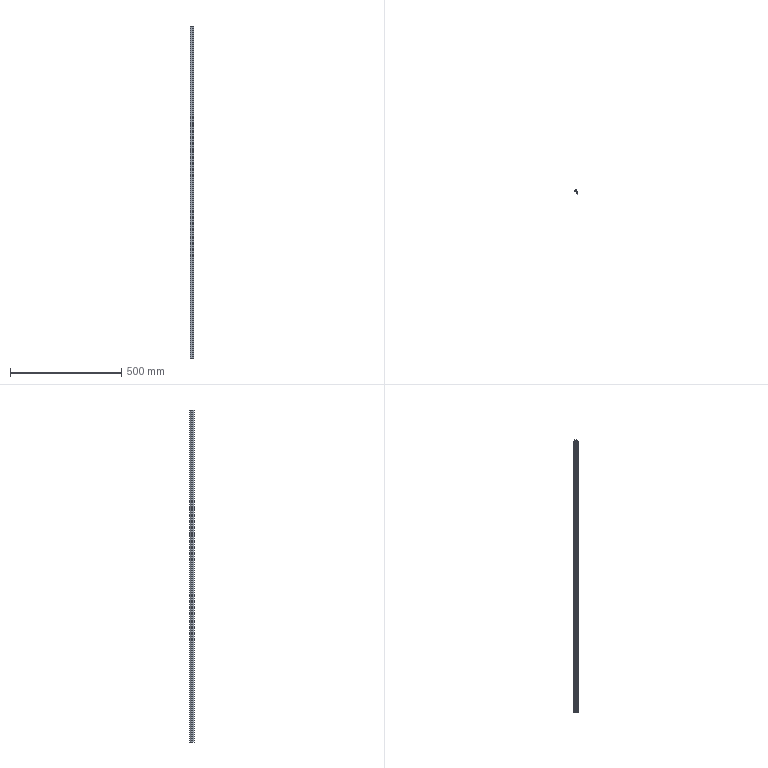Part | SolidWorks | features BaseBody 1, ICE 1, MoveFace 1 | 1 solid | 27 faces | box 14 x 20.3 x 1495 mm | volume 76119 mm3 | plane 20 | cylinder 7 | commonest cylinder face diameters 0.387 x2 0.8 x2 0.4 x1 20 x1 22 x1
STEP:
#1=CARTESIAN_POINT('',(-5.304,-0.625,200.));
#2=VERTEX_POINT('',#1);
#3=CARTESIAN_POINT('',(-5.449,-0.8125,200.));
#4=VERTEX_POINT('',#3);
#5=CARTESIAN_POINT('',(-5.255,-0.8125,200.));
#6=DIRECTION('',(0.,0.,1.));
#7=DIRECTION('',(-1.,0.,0.));
#8=AXIS2_PLACEMENT_3D('',#5,#6,#7);
#9=CIRCLE('',#8,0.1937);
#10=EDGE_CURVE('',#2,#4,#9,.T.);
#11=ORIENTED_EDGE('',*,*,#10,.T.);
#12=CARTESIAN_POINT('',(-5.449,-0.8125,-1295.));
#13=VERTEX_POINT('',#12);
#14=CARTESIAN_POINT('',(-5.449,-0.8125,230.));
#15=DIRECTION('',(0.,0.,-1.));
#16=VECTOR('',#15,1000.);
#17=LINE('',#14,#16);
#18=EDGE_CURVE('',#4,#13,#17,.T.);
#19=ORIENTED_EDGE('',*,*,#18,.T.);
#20=CARTESIAN_POINT('',(-5.304,-0.625,-1295.));
#21=VERTEX_POINT('',#20);
#22=CARTESIAN_POINT('',(-5.255,-0.8125,-1295.));
#23=DIRECTION('',(0.,0.,-1.));
#24=DIRECTION('',(1.,0.,0.));
#25=AXIS2_PLACEMENT_3D('',#22,#23,#24);
#26=CIRCLE('',#25,0.1937);
#27=EDGE_CURVE('',#13,#21,#26,.T.);
#28=ORIENTED_EDGE('',*,*,#27,.T.);
#29=CARTESIAN_POINT('',(-5.304,-0.625,230.));
#30=DIRECTION('',(0.,0.,-1.));
#31=VECTOR('',#30,1000.);
#32=LINE('',#29,#31);
#33=EDGE_CURVE('',#2,#21,#32,.T.);
#34=ORIENTED_EDGE('',*,*,#33,.F.);
#35=EDGE_LOOP('',(#11,#19,#28,#34));
#36=FACE_OUTER_BOUND('',#35,.T.);
#37=CARTESIAN_POINT('',(-5.255,-0.8125,230.));
#38=DIRECTION('',(0.,0.,-1.));
#39=DIRECTION('',(-1.,0.,0.));
#40=AXIS2_PLACEMENT_3D('',#37,#38,#39);
#41=CYLINDRICAL_SURFACE('',#40,0.1937);
#42=ADVANCED_FACE('',(#36),#41,.F.);
#43=CARTESIAN_POINT('',(5.,-1.,-1295.));
#44=VERTEX_POINT('',#43);
#45=CARTESIAN_POINT('',(5.,-14.3,-1295.));
#46=VERTEX_POINT('',#45);
#47=CARTESIAN_POINT('',(5.,29.623,-1295.));
#48=DIRECTION('',(0.,-1.,0.));
#49=VECTOR('',#48,1000.);
#50=LINE('',#47,#49);
#51=EDGE_CURVE('',#44,#46,#50,.T.);
#52=ORIENTED_EDGE('',*,*,#51,.F.);
#53=CARTESIAN_POINT('',(5.,-1.,200.));
#54=VERTEX_POINT('',#53);
#55=CARTESIAN_POINT('',(5.,-1.,230.));
#56=DIRECTION('',(0.,0.,-1.));
#57=VECTOR('',#56,1000.);
#58=LINE('',#55,#57);
#59=EDGE_CURVE('',#54,#44,#58,.T.);
#60=ORIENTED_EDGE('',*,*,#59,.F.);
#61=CARTESIAN_POINT('',(5.,-14.3,200.));
#62=VERTEX_POINT('',#61);
#63=CARTESIAN_POINT('',(5.,-14.3,200.));
#64=DIRECTION('',(0.,1.,0.));
#65=VECTOR('',#64,1000.);
#66=LINE('',#63,#65);
#67=EDGE_CURVE('',#62,#54,#66,.T.);
#68=ORIENTED_EDGE('',*,*,#67,.F.);
#69=CARTESIAN_POINT('',(5.,-14.3,230.));
#70=DIRECTION('',(0.,0.,1.));
#71=VECTOR('',#70,1000.);
#72=LINE('',#69,#71);
#73=EDGE_CURVE('',#46,#62,#72,.T.);
#74=ORIENTED_EDGE('',*,*,#73,.F.);
#75=EDGE_LOOP('',(#52,#60,#68,#74));
#76=FACE_OUTER_BOUND('',#75,.T.);
#77=CARTESIAN_POINT('',(5.,-14.3,230.));
#78=DIRECTION('',(-1.,0.,0.));
#79=DIRECTION('',(0.,0.,1.));
#80=AXIS2_PLACEMENT_3D('',#77,#78,#79);
#81=PLANE('',#80);
#82=ADVANCED_FACE('',(#76),#81,.F.);
#83=CARTESIAN_POINT('',(-9.,-2.,-1295.));
#84=VERTEX_POINT('',#83);
#85=CARTESIAN_POINT('',(-9.,-2.,200.));
#86=VERTEX_POINT('',#85);
#87=CARTESIAN_POINT('',(-9.,-2.,230.));
#88=DIRECTION('',(0.,0.,1.));
#89=VECTOR('',#88,1000.);
#90=LINE('',#87,#89);
#91=EDGE_CURVE('',#84,#86,#90,.T.);
#92=ORIENTED_EDGE('',*,*,#91,.F.);
#93=CARTESIAN_POINT('',(0.9,-2.,-1295.));
#94=VERTEX_POINT('',#93);
#95=CARTESIAN_POINT('',(5.,-2.,-1295.));
#96=DIRECTION('',(-1.,0.,0.));
#97=VECTOR('',#96,1000.);
#98=LINE('',#95,#97);
#99=EDGE_CURVE('',#94,#84,#98,.T.);
#100=ORIENTED_EDGE('',*,*,#99,.F.);
#101=CARTESIAN_POINT('',(0.9,-2.,200.));
#102=VERTEX_POINT('',#101);
#103=CARTESIAN_POINT('',(0.9,-2.,230.));
#104=DIRECTION('',(0.,0.,-1.));
#105=VECTOR('',#104,1000.);
#106=LINE('',#103,#105);
#107=EDGE_CURVE('',#102,#94,#106,.T.);
#108=ORIENTED_EDGE('',*,*,#107,.F.);
#109=CARTESIAN_POINT('',(5.,-2.,200.));
#110=DIRECTION('',(1.,0.,0.));
#111=VECTOR('',#110,1000.);
#112=LINE('',#109,#111);
#113=EDGE_CURVE('',#86,#102,#112,.T.);
#114=ORIENTED_EDGE('',*,*,#113,.F.);
#115=EDGE_LOOP('',(#92,#100,#108,#114));
#116=FACE_OUTER_BOUND('',#115,.T.);
#117=CARTESIAN_POINT('',(-9.,-2.,230.));
#118=DIRECTION('',(0.,1.,0.));
#119=DIRECTION('',(0.,0.,1.));
#120=AXIS2_PLACEMENT_3D('',#117,#118,#119);
#121=PLANE('',#120);
#122=ADVANCED_FACE('',(#116),#121,.F.);
#123=CARTESIAN_POINT('',(4.,-6.,200.));
#124=VERTEX_POINT('',#123);
#125=CARTESIAN_POINT('',(4.,-3.,200.));
#126=VERTEX_POINT('',#125);
#127=CARTESIAN_POINT('',(4.,29.623,200.));
#128=DIRECTION('',(0.,1.,0.));
#129=VECTOR('',#128,1000.);
#130=LINE('',#127,#129);
#131=EDGE_CURVE('',#124,#126,#130,.T.);
#132=ORIENTED_EDGE('',*,*,#131,.F.);
#133=CARTESIAN_POINT('',(1.,-6.,200.));
#134=VERTEX_POINT('',#133);
#135=CARTESIAN_POINT('',(5.,-6.,200.));
#136=DIRECTION('',(1.,0.,0.));
#137=VECTOR('',#136,1000.);
#138=LINE('',#135,#137);
#139=EDGE_CURVE('',#134,#124,#138,.T.);
#140=ORIENTED_EDGE('',*,*,#139,.F.);
#141=CARTESIAN_POINT('',(1.,-6.7,200.));
#142=VERTEX_POINT('',#141);
#143=CARTESIAN_POINT('',(1.,-6.,200.));
#144=DIRECTION('',(0.,-1.,0.));
#145=VECTOR('',#144,1000.);
#146=LINE('',#143,#145);
#147=EDGE_CURVE('',#134,#142,#146,.T.);
#148=ORIENTED_EDGE('',*,*,#147,.T.);
#149=CARTESIAN_POINT('',(-1.7,-6.7,200.));
#150=VERTEX_POINT('',#149);
#151=CARTESIAN_POINT('',(5.,-6.7,200.));
#152=DIRECTION('',(1.,0.,0.));
#153=VECTOR('',#152,1000.);
#154=LINE('',#151,#153);
#155=EDGE_CURVE('',#150,#142,#154,.T.);
#156=ORIENTED_EDGE('',*,*,#155,.F.);
#157=CARTESIAN_POINT('',(-1.7,-7.7,200.));
#158=VERTEX_POINT('',#157);
#159=CARTESIAN_POINT('',(-1.7,-6.7,200.));
#160=DIRECTION('',(0.,-1.,0.));
#161=VECTOR('',#160,1000.);
#162=LINE('',#159,#161);
#163=EDGE_CURVE('',#150,#158,#162,.T.);
#164=ORIENTED_EDGE('',*,*,#163,.T.);
#165=CARTESIAN_POINT('',(4.,-7.7,200.));
#166=VERTEX_POINT('',#165);
#167=CARTESIAN_POINT('',(5.,-7.7,200.));
#168=DIRECTION('',(-1.,0.,0.));
#169=VECTOR('',#168,1000.);
#170=LINE('',#167,#169);
#171=EDGE_CURVE('',#166,#158,#170,.T.);
#172=ORIENTED_EDGE('',*,*,#171,.F.);
#173=CARTESIAN_POINT('',(4.,-14.3,200.));
#174=VERTEX_POINT('',#173);
#175=CARTESIAN_POINT('',(4.,29.623,200.));
#176=DIRECTION('',(0.,1.,0.));
#177=VECTOR('',#176,1000.);
#178=LINE('',#175,#177);
#179=EDGE_CURVE('',#174,#166,#178,.T.);
#180=ORIENTED_EDGE('',*,*,#179,.F.);
#181=CARTESIAN_POINT('',(5.,-14.3,200.));
#182=DIRECTION('',(-1.,0.,0.));
#183=VECTOR('',#182,1000.);
#184=LINE('',#181,#183);
#185=EDGE_CURVE('',#62,#174,#184,.T.);
#186=ORIENTED_EDGE('',*,*,#185,.F.);
#187=ORIENTED_EDGE('',*,*,#67,.T.);
#188=CARTESIAN_POINT('',(-5.207,-1.,200.));
#189=VERTEX_POINT('',#188);
#190=CARTESIAN_POINT('',(5.,-1.,200.));
#191=DIRECTION('',(1.,0.,0.));
#192=VECTOR('',#191,1000.);
#193=LINE('',#190,#192);
#194=EDGE_CURVE('',#189,#54,#193,.T.);
#195=ORIENTED_EDGE('',*,*,#194,.F.);
#196=CARTESIAN_POINT('',(-5.255,-0.8125,200.));
#197=DIRECTION('',(0.,0.,1.));
#198=DIRECTION('',(-1.,0.,0.));
#199=AXIS2_PLACEMENT_3D('',#196,#197,#198);
#200=CIRCLE('',#199,0.1937);
#201=EDGE_CURVE('',#4,#189,#200,.T.);
#202=ORIENTED_EDGE('',*,*,#201,.F.);
#203=ORIENTED_EDGE('',*,*,#10,.F.);
#204=CARTESIAN_POINT('',(-1.368,3.063,200.));
#205=VERTEX_POINT('',#204);
#206=CARTESIAN_POINT('',(-10.628,9.,200.));
#207=DIRECTION('',(0.,0.,1.));
#208=DIRECTION('',(-1.,0.,0.));
#209=AXIS2_PLACEMENT_3D('',#206,#207,#208);
#210=CIRCLE('',#209,11.);
#211=EDGE_CURVE('',#2,#205,#210,.T.);
#212=ORIENTED_EDGE('',*,*,#211,.T.);
#213=CARTESIAN_POINT('',(-1.,2.955,200.));
#214=VERTEX_POINT('',#213);
#215=CARTESIAN_POINT('',(-1.2,2.955,200.));
#216=DIRECTION('',(0.,0.,1.));
#217=DIRECTION('',(-1.,0.,0.));
#218=AXIS2_PLACEMENT_3D('',#215,#216,#217);
#219=CIRCLE('',#218,0.2);
#220=EDGE_CURVE('',#214,#205,#219,.T.);
#221=ORIENTED_EDGE('',*,*,#220,.F.);
#222=CARTESIAN_POINT('',(-1.,1.5,200.));
#223=VERTEX_POINT('',#222);
#224=CARTESIAN_POINT('',(-1.,2.955,200.));
#225=DIRECTION('',(0.,1.,0.));
#226=VECTOR('',#225,1000.);
#227=LINE('',#224,#226);
#228=EDGE_CURVE('',#223,#214,#227,.T.);
#229=ORIENTED_EDGE('',*,*,#228,.F.);
#230=CARTESIAN_POINT('',(0.,1.5,200.));
#231=VERTEX_POINT('',#230);
#232=CARTESIAN_POINT('',(-1.,1.5,200.));
#233=DIRECTION('',(-1.,0.,0.));
#234=VECTOR('',#233,1000.);
#235=LINE('',#232,#234);
#236=EDGE_CURVE('',#231,#223,#235,.T.);
#237=ORIENTED_EDGE('',*,*,#236,.F.);
#238=CARTESIAN_POINT('',(0.,6.,200.));
#239=VERTEX_POINT('',#238);
#240=CARTESIAN_POINT('',(0.,1.5,200.));
#241=DIRECTION('',(0.,-1.,0.));
#242=VECTOR('',#241,1000.);
#243=LINE('',#240,#242);
#244=EDGE_CURVE('',#239,#231,#243,.T.);
#245=ORIENTED_EDGE('',*,*,#244,.F.);
#246=CARTESIAN_POINT('',(-0.8,6.,200.));
#247=VERTEX_POINT('',#246);
#248=CARTESIAN_POINT('',(0.,6.,200.));
#249=DIRECTION('',(1.,0.,0.));
#250=VECTOR('',#249,1000.);
#251=LINE('',#248,#250);
#252=EDGE_CURVE('',#247,#239,#251,.T.);
#253=ORIENTED_EDGE('',*,*,#252,.F.);
#254=CARTESIAN_POINT('',(-1.178,5.731,200.));
#255=VERTEX_POINT('',#254);
#256=CARTESIAN_POINT('',(-0.8,5.6,200.));
#257=DIRECTION('',(0.,0.,1.));
#258=DIRECTION('',(-1.,0.,0.));
#259=AXIS2_PLACEMENT_3D('',#256,#257,#258);
#260=CIRCLE('',#259,0.4);
#261=EDGE_CURVE('',#247,#255,#260,.T.);
#262=ORIENTED_EDGE('',*,*,#261,.T.);
#263=CARTESIAN_POINT('',(-8.678,-0.8077,200.));
#264=VERTEX_POINT('',#263);
#265=CARTESIAN_POINT('',(-10.628,9.,200.));
#266=DIRECTION('',(0.,0.,1.));
#267=DIRECTION('',(-1.,0.,0.));
#268=AXIS2_PLACEMENT_3D('',#265,#266,#267);
#269=CIRCLE('',#268,10.);
#270=EDGE_CURVE('',#264,#255,#269,.T.);
#271=ORIENTED_EDGE('',*,*,#270,.F.);
#272=CARTESIAN_POINT('',(-9.,-1.2,200.));
#273=VERTEX_POINT('',#272);
#274=CARTESIAN_POINT('',(-8.6,-1.2,200.));
#275=DIRECTION('',(0.,0.,1.));
#276=DIRECTION('',(-1.,0.,0.));
#277=AXIS2_PLACEMENT_3D('',#274,#275,#276);
#278=CIRCLE('',#277,0.4);
#279=EDGE_CURVE('',#264,#273,#278,.T.);
#280=ORIENTED_EDGE('',*,*,#279,.T.);
#281=CARTESIAN_POINT('',(-9.,8.,200.));
#282=DIRECTION('',(0.,-1.,0.));
#283=VECTOR('',#282,1000.);
#284=LINE('',#281,#283);
#285=EDGE_CURVE('',#273,#86,#284,.T.);
#286=ORIENTED_EDGE('',*,*,#285,.T.);
#287=ORIENTED_EDGE('',*,*,#113,.T.);
#288=CARTESIAN_POINT('',(0.9,-3.,200.));
#289=VERTEX_POINT('',#288);
#290=CARTESIAN_POINT('',(0.9,29.623,200.));
#291=DIRECTION('',(0.,1.,0.));
#292=VECTOR('',#291,1000.);
#293=LINE('',#290,#292);
#294=EDGE_CURVE('',#289,#102,#293,.T.);
#295=ORIENTED_EDGE('',*,*,#294,.F.);
#296=CARTESIAN_POINT('',(5.,-3.,200.));
#297=DIRECTION('',(-1.,0.,0.));
#298=VECTOR('',#297,1000.);
#299=LINE('',#296,#298);
#300=EDGE_CURVE('',#126,#289,#299,.T.);
#301=ORIENTED_EDGE('',*,*,#300,.F.);
#302=EDGE_LOOP('',(#132,#140,#148,#156,#164,#172,#180,#186,#187,#195,#202,#203,#212,#221,#229,#237,#245,#253,#262,#271,#280,#286,#287,#295,#301));
#303=FACE_OUTER_BOUND('',#302,.T.);
#304=CARTESIAN_POINT('',(5.,29.623,200.));
#305=DIRECTION('',(0.,0.,-1.));
#306=DIRECTION('',(-1.,0.,0.));
#307=AXIS2_PLACEMENT_3D('',#304,#305,#306);
#308=PLANE('',#307);
#309=ADVANCED_FACE('',(#303),#308,.F.);
#310=ORIENTED_EDGE('',*,*,#185,.T.);
#311=CARTESIAN_POINT('',(4.,-14.3,-1295.));
#312=VERTEX_POINT('',#311);
#313=CARTESIAN_POINT('',(4.,-14.3,230.));
#314=DIRECTION('',(0.,0.,1.));
#315=VECTOR('',#314,1000.);
#316=LINE('',#313,#315);
#317=EDGE_CURVE('',#312,#174,#316,.T.);
#318=ORIENTED_EDGE('',*,*,#317,.F.);
#319=CARTESIAN_POINT('',(5.,-14.3,-1295.));
#320=DIRECTION('',(-1.,0.,0.));
#321=VECTOR('',#320,1000.);
#322=LINE('',#319,#321);
#323=EDGE_CURVE('',#46,#312,#322,.T.);
#324=ORIENTED_EDGE('',*,*,#323,.F.);
#325=ORIENTED_EDGE('',*,*,#73,.T.);
#326=EDGE_LOOP('',(#310,#318,#324,#325));
#327=FACE_OUTER_BOUND('',#326,.T.);
#328=CARTESIAN_POINT('',(4.,-14.3,230.));
#329=DIRECTION('',(0.,1.,0.));
#330=DIRECTION('',(0.,0.,1.));
#331=AXIS2_PLACEMENT_3D('',#328,#329,#330);
#332=PLANE('',#331);
#333=ADVANCED_FACE('',(#327),#332,.F.);
#334=ORIENTED_EDGE('',*,*,#51,.T.);
#335=ORIENTED_EDGE('',*,*,#323,.T.);
#336=CARTESIAN_POINT('',(4.,-7.7,-1295.));
#337=VERTEX_POINT('',#336);
#338=CARTESIAN_POINT('',(4.,-7.7,-1295.));
#339=DIRECTION('',(0.,-1.,0.));
#340=VECTOR('',#339,1000.);
#341=LINE('',#338,#340);
#342=EDGE_CURVE('',#337,#312,#341,.T.);
#343=ORIENTED_EDGE('',*,*,#342,.F.);
#344=CARTESIAN_POINT('',(-1.7,-7.7,-1295.));
#345=VERTEX_POINT('',#344);
#346=CARTESIAN_POINT('',(-1.7,-7.7,-1295.));
#347=DIRECTION('',(1.,0.,0.));
#348=VECTOR('',#347,1000.);
#349=LINE('',#346,#348);
#350=EDGE_CURVE('',#345,#337,#349,.T.);
#351=ORIENTED_EDGE('',*,*,#350,.F.);
#352=CARTESIAN_POINT('',(-1.7,-6.7,-1295.));
#353=VERTEX_POINT('',#352);
#354=CARTESIAN_POINT('',(-1.7,29.623,-1295.));
#355=DIRECTION('',(0.,1.,0.));
#356=VECTOR('',#355,1000.);
#357=LINE('',#354,#356);
#358=EDGE_CURVE('',#345,#353,#357,.T.);
#359=ORIENTED_EDGE('',*,*,#358,.T.);
#360=CARTESIAN_POINT('',(1.,-6.7,-1295.));
#361=VERTEX_POINT('',#360);
#362=CARTESIAN_POINT('',(1.,-6.7,-1295.));
#363=DIRECTION('',(-1.,0.,0.));
#364=VECTOR('',#363,1000.);
#365=LINE('',#362,#364);
#366=EDGE_CURVE('',#361,#353,#365,.T.);
#367=ORIENTED_EDGE('',*,*,#366,.F.);
#368=CARTESIAN_POINT('',(1.,-6.,-1295.));
#369=VERTEX_POINT('',#368);
#370=CARTESIAN_POINT('',(1.,29.623,-1295.));
#371=DIRECTION('',(0.,1.,0.));
#372=VECTOR('',#371,1000.);
#373=LINE('',#370,#372);
#374=EDGE_CURVE('',#361,#369,#373,.T.);
#375=ORIENTED_EDGE('',*,*,#374,.T.);
#376=CARTESIAN_POINT('',(4.,-6.,-1295.));
#377=VERTEX_POINT('',#376);
#378=CARTESIAN_POINT('',(4.,-6.,-1295.));
#379=DIRECTION('',(-1.,0.,0.));
#380=VECTOR('',#379,1000.);
#381=LINE('',#378,#380);
#382=EDGE_CURVE('',#377,#369,#381,.T.);
#383=ORIENTED_EDGE('',*,*,#382,.F.);
#384=CARTESIAN_POINT('',(4.,-3.,-1295.));
#385=VERTEX_POINT('',#384);
#386=CARTESIAN_POINT('',(4.,-3.,-1295.));
#387=DIRECTION('',(0.,-1.,0.));
#388=VECTOR('',#387,1000.);
#389=LINE('',#386,#388);
#390=EDGE_CURVE('',#385,#377,#389,.T.);
#391=ORIENTED_EDGE('',*,*,#390,.F.);
#392=CARTESIAN_POINT('',(0.9,-3.,-1295.));
#393=VERTEX_POINT('',#392);
#394=CARTESIAN_POINT('',(0.9,-3.,-1295.));
#395=DIRECTION('',(1.,0.,0.));
#396=VECTOR('',#395,1000.);
#397=LINE('',#394,#396);
#398=EDGE_CURVE('',#393,#385,#397,.T.);
#399=ORIENTED_EDGE('',*,*,#398,.F.);
#400=CARTESIAN_POINT('',(0.9,-2.,-1295.));
#401=DIRECTION('',(0.,-1.,0.));
#402=VECTOR('',#401,1000.);
#403=LINE('',#400,#402);
#404=EDGE_CURVE('',#94,#393,#403,.T.);
#405=ORIENTED_EDGE('',*,*,#404,.F.);
#406=ORIENTED_EDGE('',*,*,#99,.T.);
#407=CARTESIAN_POINT('',(-9.,-1.2,-1295.));
#408=VERTEX_POINT('',#407);
#409=CARTESIAN_POINT('',(-9.,-1.2,-1295.));
#410=DIRECTION('',(0.,-1.,0.));
#411=VECTOR('',#410,1000.);
#412=LINE('',#409,#411);
#413=EDGE_CURVE('',#408,#84,#412,.T.);
#414=ORIENTED_EDGE('',*,*,#413,.F.);
#415=CARTESIAN_POINT('',(-8.678,-0.8077,-1295.));
#416=VERTEX_POINT('',#415);
#417=CARTESIAN_POINT('',(-8.6,-1.2,-1295.));
#418=DIRECTION('',(0.,0.,-1.));
#419=DIRECTION('',(1.,0.,0.));
#420=AXIS2_PLACEMENT_3D('',#417,#418,#419);
#421=CIRCLE('',#420,0.4);
#422=EDGE_CURVE('',#408,#416,#421,.T.);
#423=ORIENTED_EDGE('',*,*,#422,.T.);
#424=CARTESIAN_POINT('',(-1.178,5.731,-1295.));
#425=VERTEX_POINT('',#424);
#426=CARTESIAN_POINT('',(-10.628,9.,-1295.));
#427=DIRECTION('',(0.,0.,-1.));
#428=DIRECTION('',(1.,0.,0.));
#429=AXIS2_PLACEMENT_3D('',#426,#427,#428);
#430=CIRCLE('',#429,10.);
#431=EDGE_CURVE('',#425,#416,#430,.T.);
#432=ORIENTED_EDGE('',*,*,#431,.F.);
#433=CARTESIAN_POINT('',(-0.8,6.,-1295.));
#434=VERTEX_POINT('',#433);
#435=CARTESIAN_POINT('',(-0.8,5.6,-1295.));
#436=DIRECTION('',(0.,0.,-1.));
#437=DIRECTION('',(1.,0.,0.));
#438=AXIS2_PLACEMENT_3D('',#435,#436,#437);
#439=CIRCLE('',#438,0.4);
#440=EDGE_CURVE('',#425,#434,#439,.T.);
#441=ORIENTED_EDGE('',*,*,#440,.T.);
#442=CARTESIAN_POINT('',(0.,6.,-1295.));
#443=VERTEX_POINT('',#442);
#444=CARTESIAN_POINT('',(0.,6.,-1295.));
#445=DIRECTION('',(-1.,0.,0.));
#446=VECTOR('',#445,1000.);
#447=LINE('',#444,#446);
#448=EDGE_CURVE('',#443,#434,#447,.T.);
#449=ORIENTED_EDGE('',*,*,#448,.F.);
#450=CARTESIAN_POINT('',(0.,1.5,-1295.));
#451=VERTEX_POINT('',#450);
#452=CARTESIAN_POINT('',(0.,1.5,-1295.));
#453=DIRECTION('',(0.,1.,0.));
#454=VECTOR('',#453,1000.);
#455=LINE('',#452,#454);
#456=EDGE_CURVE('',#451,#443,#455,.T.);
#457=ORIENTED_EDGE('',*,*,#456,.F.);
#458=CARTESIAN_POINT('',(-1.,1.5,-1295.));
#459=VERTEX_POINT('',#458);
#460=CARTESIAN_POINT('',(-1.,1.5,-1295.));
#461=DIRECTION('',(1.,0.,0.));
#462=VECTOR('',#461,1000.);
#463=LINE('',#460,#462);
#464=EDGE_CURVE('',#459,#451,#463,.T.);
#465=ORIENTED_EDGE('',*,*,#464,.F.);
#466=CARTESIAN_POINT('',(-1.,2.955,-1295.));
#467=VERTEX_POINT('',#466);
#468=CARTESIAN_POINT('',(-1.,2.955,-1295.));
#469=DIRECTION('',(0.,-1.,0.));
#470=VECTOR('',#469,1000.);
#471=LINE('',#468,#470);
#472=EDGE_CURVE('',#467,#459,#471,.T.);
#473=ORIENTED_EDGE('',*,*,#472,.F.);
#474=CARTESIAN_POINT('',(-1.368,3.063,-1295.));
#475=VERTEX_POINT('',#474);
#476=CARTESIAN_POINT('',(-1.2,2.955,-1295.));
#477=DIRECTION('',(0.,0.,-1.));
#478=DIRECTION('',(1.,0.,0.));
#479=AXIS2_PLACEMENT_3D('',#476,#477,#478);
#480=CIRCLE('',#479,0.2);
#481=EDGE_CURVE('',#475,#467,#480,.T.);
#482=ORIENTED_EDGE('',*,*,#481,.F.);
#483=CARTESIAN_POINT('',(-10.628,9.,-1295.));
#484=DIRECTION('',(0.,0.,-1.));
#485=DIRECTION('',(1.,0.,0.));
#486=AXIS2_PLACEMENT_3D('',#483,#484,#485);
#487=CIRCLE('',#486,11.);
#488=EDGE_CURVE('',#475,#21,#487,.T.);
#489=ORIENTED_EDGE('',*,*,#488,.T.);
#490=ORIENTED_EDGE('',*,*,#27,.F.);
#491=CARTESIAN_POINT('',(-5.207,-1.,-1295.));
#492=VERTEX_POINT('',#491);
#493=CARTESIAN_POINT('',(-5.255,-0.8125,-1295.));
#494=DIRECTION('',(0.,0.,-1.));
#495=DIRECTION('',(1.,0.,0.));
#496=AXIS2_PLACEMENT_3D('',#493,#494,#495);
#497=CIRCLE('',#496,0.1937);
#498=EDGE_CURVE('',#492,#13,#497,.T.);
#499=ORIENTED_EDGE('',*,*,#498,.F.);
#500=CARTESIAN_POINT('',(5.,-1.,-1295.));
#501=DIRECTION('',(-1.,0.,0.));
#502=VECTOR('',#501,1000.);
#503=LINE('',#500,#502);
#504=EDGE_CURVE('',#44,#492,#503,.T.);
#505=ORIENTED_EDGE('',*,*,#504,.F.);
#506=EDGE_LOOP('',(#334,#335,#343,#351,#359,#367,#375,#383,#391,#399,#405,#406,#414,#423,#432,#441,#449,#457,#465,#473,#482,#489,#490,#499,#505));
#507=FACE_OUTER_BOUND('',#506,.T.);
#508=CARTESIAN_POINT('',(5.,29.623,-1295.));
#509=DIRECTION('',(0.,0.,1.));
#510=DIRECTION('',(1.,0.,0.));
#511=AXIS2_PLACEMENT_3D('',#508,#509,#510);
#512=PLANE('',#511);
#513=ADVANCED_FACE('',(#507),#512,.F.);
#514=ORIENTED_EDGE('',*,*,#59,.T.);
#515=ORIENTED_EDGE('',*,*,#504,.T.);
#516=CARTESIAN_POINT('',(-5.207,-1.,230.));
#517=DIRECTION('',(0.,0.,-1.));
#518=VECTOR('',#517,1000.);
#519=LINE('',#516,#518);
#520=EDGE_CURVE('',#189,#492,#519,.T.);
#521=ORIENTED_EDGE('',*,*,#520,.F.);
#522=ORIENTED_EDGE('',*,*,#194,.T.);
#523=EDGE_LOOP('',(#514,#515,#521,#522));
#524=FACE_OUTER_BOUND('',#523,.T.);
#525=CARTESIAN_POINT('',(5.,-1.,230.));
#526=DIRECTION('',(0.,-1.,0.));
#527=DIRECTION('',(0.,0.,-1.));
#528=AXIS2_PLACEMENT_3D('',#525,#526,#527);
#529=PLANE('',#528);
#530=ADVANCED_FACE('',(#524),#529,.F.);
#531=CARTESIAN_POINT('',(-9.,-1.2,230.));
#532=DIRECTION('',(0.,0.,1.));
#533=VECTOR('',#532,1000.);
#534=LINE('',#531,#533);
#535=EDGE_CURVE('',#408,#273,#534,.T.);
#536=ORIENTED_EDGE('',*,*,#535,.F.);
#537=ORIENTED_EDGE('',*,*,#413,.T.);
#538=ORIENTED_EDGE('',*,*,#91,.T.);
#539=ORIENTED_EDGE('',*,*,#285,.F.);
#540=EDGE_LOOP('',(#536,#537,#538,#539));
#541=FACE_OUTER_BOUND('',#540,.T.);
#542=CARTESIAN_POINT('',(-9.,-1.2,230.));
#543=DIRECTION('',(1.,0.,0.));
#544=DIRECTION('',(0.,0.,-1.));
#545=AXIS2_PLACEMENT_3D('',#542,#543,#544);
#546=PLANE('',#545);
#547=ADVANCED_FACE('',(#541),#546,.F.);
#548=ORIENTED_EDGE('',*,*,#294,.T.);
#549=ORIENTED_EDGE('',*,*,#107,.T.);
#550=ORIENTED_EDGE('',*,*,#404,.T.);
#551=CARTESIAN_POINT('',(0.9,-3.,230.));
#552=DIRECTION('',(0.,0.,-1.));
#553=VECTOR('',#552,1000.);
#554=LINE('',#551,#553);
#555=EDGE_CURVE('',#289,#393,#554,.T.);
#556=ORIENTED_EDGE('',*,*,#555,.F.);
#557=EDGE_LOOP('',(#548,#549,#550,#556));
#558=FACE_OUTER_BOUND('',#557,.T.);
#559=CARTESIAN_POINT('',(0.9,-2.,230.));
#560=DIRECTION('',(1.,0.,0.));
#561=DIRECTION('',(0.,0.,-1.));
#562=AXIS2_PLACEMENT_3D('',#559,#560,#561);
#563=PLANE('',#562);
#564=ADVANCED_FACE('',(#558),#563,.F.);
#565=ORIENTED_EDGE('',*,*,#300,.T.);
#566=ORIENTED_EDGE('',*,*,#555,.T.);
#567=ORIENTED_EDGE('',*,*,#398,.T.);
#568=CARTESIAN_POINT('',(4.,-3.,230.));
#569=DIRECTION('',(0.,0.,-1.));
#570=VECTOR('',#569,1000.);
#571=LINE('',#568,#570);
#572=EDGE_CURVE('',#126,#385,#571,.T.);
#573=ORIENTED_EDGE('',*,*,#572,.F.);
#574=EDGE_LOOP('',(#565,#566,#567,#573));
#575=FACE_OUTER_BOUND('',#574,.T.);
#576=CARTESIAN_POINT('',(0.9,-3.,230.));
#577=DIRECTION('',(0.,1.,0.));
#578=DIRECTION('',(0.,0.,1.));
#579=AXIS2_PLACEMENT_3D('',#576,#577,#578);
#580=PLANE('',#579);
#581=ADVANCED_FACE('',(#575),#580,.F.);
#582=ORIENTED_EDGE('',*,*,#131,.T.);
#583=ORIENTED_EDGE('',*,*,#572,.T.);
#584=ORIENTED_EDGE('',*,*,#390,.T.);
#585=CARTESIAN_POINT('',(4.,-6.,230.));
#586=DIRECTION('',(0.,0.,-1.));
#587=VECTOR('',#586,1000.);
#588=LINE('',#585,#587);
#589=EDGE_CURVE('',#124,#377,#588,.T.);
#590=ORIENTED_EDGE('',*,*,#589,.F.);
#591=EDGE_LOOP('',(#582,#583,#584,#590));
#592=FACE_OUTER_BOUND('',#591,.T.);
#593=CARTESIAN_POINT('',(4.,-3.,230.));
#594=DIRECTION('',(1.,0.,0.));
#595=DIRECTION('',(0.,0.,-1.));
#596=AXIS2_PLACEMENT_3D('',#593,#594,#595);
#597=PLANE('',#596);
#598=ADVANCED_FACE('',(#592),#597,.F.);
#599=ORIENTED_EDGE('',*,*,#139,.T.);
#600=ORIENTED_EDGE('',*,*,#589,.T.);
#601=ORIENTED_EDGE('',*,*,#382,.T.);
#602=CARTESIAN_POINT('',(1.,-6.,230.));
#603=DIRECTION('',(0.,0.,-1.));
#604=VECTOR('',#603,1000.);
#605=LINE('',#602,#604);
#606=EDGE_CURVE('',#134,#369,#605,.T.);
#607=ORIENTED_EDGE('',*,*,#606,.F.);
#608=EDGE_LOOP('',(#599,#600,#601,#607));
#609=FACE_OUTER_BOUND('',#608,.T.);
#610=CARTESIAN_POINT('',(4.,-6.,230.));
#611=DIRECTION('',(0.,-1.,0.));
#612=DIRECTION('',(0.,0.,-1.));
#613=AXIS2_PLACEMENT_3D('',#610,#611,#612);
#614=PLANE('',#613);
#615=ADVANCED_FACE('',(#609),#614,.F.);
#616=ORIENTED_EDGE('',*,*,#155,.T.);
#617=CARTESIAN_POINT('',(1.,-6.7,230.));
#618=DIRECTION('',(0.,0.,1.));
#619=VECTOR('',#618,1000.);
#620=LINE('',#617,#619);
#621=EDGE_CURVE('',#361,#142,#620,.T.);
#622=ORIENTED_EDGE('',*,*,#621,.F.);
#623=ORIENTED_EDGE('',*,*,#366,.T.);
#624=CARTESIAN_POINT('',(-1.7,-6.7,230.));
#625=DIRECTION('',(0.,0.,-1.));
#626=VECTOR('',#625,1000.);
#627=LINE('',#624,#626);
#628=EDGE_CURVE('',#150,#353,#627,.T.);
#629=ORIENTED_EDGE('',*,*,#628,.F.);
#630=EDGE_LOOP('',(#616,#622,#623,#629));
#631=FACE_OUTER_BOUND('',#630,.T.);
#632=CARTESIAN_POINT('',(1.,-6.7,230.));
#633=DIRECTION('',(0.,-1.,0.));
#634=DIRECTION('',(0.,0.,-1.));
#635=AXIS2_PLACEMENT_3D('',#632,#633,#634);
#636=PLANE('',#635);
#637=ADVANCED_FACE('',(#631),#636,.F.);
#638=ORIENTED_EDGE('',*,*,#171,.T.);
#639=CARTESIAN_POINT('',(-1.7,-7.7,230.));
#640=DIRECTION('',(0.,0.,1.));
#641=VECTOR('',#640,1000.);
#642=LINE('',#639,#641);
#643=EDGE_CURVE('',#345,#158,#642,.T.);
#644=ORIENTED_EDGE('',*,*,#643,.F.);
#645=ORIENTED_EDGE('',*,*,#350,.T.);
#646=CARTESIAN_POINT('',(4.,-7.7,230.));
#647=DIRECTION('',(0.,0.,-1.));
#648=VECTOR('',#647,1000.);
#649=LINE('',#646,#648);
#650=EDGE_CURVE('',#166,#337,#649,.T.);
#651=ORIENTED_EDGE('',*,*,#650,.F.);
#652=EDGE_LOOP('',(#638,#644,#645,#651));
#653=FACE_OUTER_BOUND('',#652,.T.);
#654=CARTESIAN_POINT('',(-1.7,-7.7,230.));
#655=DIRECTION('',(0.,1.,0.));
#656=DIRECTION('',(0.,0.,1.));
#657=AXIS2_PLACEMENT_3D('',#654,#655,#656);
#658=PLANE('',#657);
#659=ADVANCED_FACE('',(#653),#658,.F.);
#660=ORIENTED_EDGE('',*,*,#179,.T.);
#661=ORIENTED_EDGE('',*,*,#650,.T.);
#662=ORIENTED_EDGE('',*,*,#342,.T.);
#663=ORIENTED_EDGE('',*,*,#317,.T.);
#664=EDGE_LOOP('',(#660,#661,#662,#663));
#665=FACE_OUTER_BOUND('',#664,.T.);
#666=CARTESIAN_POINT('',(4.,-7.7,230.));
#667=DIRECTION('',(1.,0.,0.));
#668=DIRECTION('',(0.,0.,-1.));
#669=AXIS2_PLACEMENT_3D('',#666,#667,#668);
#670=PLANE('',#669);
#671=ADVANCED_FACE('',(#665),#670,.F.);
#672=ORIENTED_EDGE('',*,*,#18,.F.);
#673=ORIENTED_EDGE('',*,*,#201,.T.);
#674=ORIENTED_EDGE('',*,*,#520,.T.);
#675=ORIENTED_EDGE('',*,*,#498,.T.);
#676=EDGE_LOOP('',(#672,#673,#674,#675));
#677=FACE_OUTER_BOUND('',#676,.T.);
#678=CARTESIAN_POINT('',(-5.255,-0.8125,230.));
#679=DIRECTION('',(0.,0.,-1.));
#680=DIRECTION('',(-1.,0.,0.));
#681=AXIS2_PLACEMENT_3D('',#678,#679,#680);
#682=CYLINDRICAL_SURFACE('',#681,0.1937);
#683=ADVANCED_FACE('',(#677),#682,.F.);
#684=CARTESIAN_POINT('',(-1.,2.955,230.));
#685=DIRECTION('',(0.,0.,1.));
#686=VECTOR('',#685,1000.);
#687=LINE('',#684,#686);
#688=EDGE_CURVE('',#467,#214,#687,.T.);
#689=ORIENTED_EDGE('',*,*,#688,.F.);
#690=ORIENTED_EDGE('',*,*,#472,.T.);
#691=CARTESIAN_POINT('',(-1.,1.5,230.));
#692=DIRECTION('',(0.,0.,-1.));
#693=VECTOR('',#692,1000.);
#694=LINE('',#691,#693);
#695=EDGE_CURVE('',#223,#459,#694,.T.);
#696=ORIENTED_EDGE('',*,*,#695,.F.);
#697=ORIENTED_EDGE('',*,*,#228,.T.);
#698=EDGE_LOOP('',(#689,#690,#696,#697));
#699=FACE_OUTER_BOUND('',#698,.T.);
#700=CARTESIAN_POINT('',(-1.,2.955,230.));
#701=DIRECTION('',(1.,0.,0.));
#702=DIRECTION('',(0.,0.,-1.));
#703=AXIS2_PLACEMENT_3D('',#700,#701,#702);
#704=PLANE('',#703);
#705=ADVANCED_FACE('',(#699),#704,.F.);
#706=ORIENTED_EDGE('',*,*,#488,.F.);
#707=CARTESIAN_POINT('',(-1.368,3.063,230.));
#708=DIRECTION('',(0.,0.,1.));
#709=VECTOR('',#708,1000.);
#710=LINE('',#707,#709);
#711=EDGE_CURVE('',#475,#205,#710,.T.);
#712=ORIENTED_EDGE('',*,*,#711,.T.);
#713=ORIENTED_EDGE('',*,*,#211,.F.);
#714=ORIENTED_EDGE('',*,*,#33,.T.);
#715=EDGE_LOOP('',(#706,#712,#713,#714));
#716=FACE_OUTER_BOUND('',#715,.T.);
#717=CARTESIAN_POINT('',(-10.628,9.,230.));
#718=DIRECTION('',(0.,0.,-1.));
#719=DIRECTION('',(-1.,0.,0.));
#720=AXIS2_PLACEMENT_3D('',#717,#718,#719);
#721=CYLINDRICAL_SURFACE('',#720,11.);
#722=ADVANCED_FACE('',(#716),#721,.T.);
#723=CARTESIAN_POINT('',(-1.178,5.731,230.));
#724=DIRECTION('',(0.,0.,1.));
#725=VECTOR('',#724,1000.);
#726=LINE('',#723,#725);
#727=EDGE_CURVE('',#425,#255,#726,.T.);
#728=ORIENTED_EDGE('',*,*,#727,.F.);
#729=ORIENTED_EDGE('',*,*,#431,.T.);
#730=CARTESIAN_POINT('',(-8.678,-0.8077,230.));
#731=DIRECTION('',(0.,0.,-1.));
#732=VECTOR('',#731,1000.);
#733=LINE('',#730,#732);
#734=EDGE_CURVE('',#264,#416,#733,.T.);
#735=ORIENTED_EDGE('',*,*,#734,.F.);
#736=ORIENTED_EDGE('',*,*,#270,.T.);
#737=EDGE_LOOP('',(#728,#729,#735,#736));
#738=FACE_OUTER_BOUND('',#737,.T.);
#739=CARTESIAN_POINT('',(-10.628,9.,230.));
#740=DIRECTION('',(0.,0.,-1.));
#741=DIRECTION('',(-1.,0.,0.));
#742=AXIS2_PLACEMENT_3D('',#739,#740,#741);
#743=CYLINDRICAL_SURFACE('',#742,10.);
#744=ADVANCED_FACE('',(#738),#743,.F.);
#745=CARTESIAN_POINT('',(0.,1.5,230.));
#746=DIRECTION('',(0.,0.,1.));
#747=VECTOR('',#746,1000.);
#748=LINE('',#745,#747);
#749=EDGE_CURVE('',#451,#231,#748,.T.);
#750=ORIENTED_EDGE('',*,*,#749,.F.);
#751=ORIENTED_EDGE('',*,*,#456,.T.);
#752=CARTESIAN_POINT('',(0.,6.,230.));
#753=DIRECTION('',(0.,0.,-1.));
#754=VECTOR('',#753,1000.);
#755=LINE('',#752,#754);
#756=EDGE_CURVE('',#239,#443,#755,.T.);
#757=ORIENTED_EDGE('',*,*,#756,.F.);
#758=ORIENTED_EDGE('',*,*,#244,.T.);
#759=EDGE_LOOP('',(#750,#751,#757,#758));
#760=FACE_OUTER_BOUND('',#759,.T.);
#761=CARTESIAN_POINT('',(0.,1.5,230.));
#762=DIRECTION('',(-1.,0.,0.));
#763=DIRECTION('',(0.,0.,1.));
#764=AXIS2_PLACEMENT_3D('',#761,#762,#763);
#765=PLANE('',#764);
#766=ADVANCED_FACE('',(#760),#765,.F.);
#767=ORIENTED_EDGE('',*,*,#422,.F.);
#768=ORIENTED_EDGE('',*,*,#535,.T.);
#769=ORIENTED_EDGE('',*,*,#279,.F.);
#770=ORIENTED_EDGE('',*,*,#734,.T.);
#771=EDGE_LOOP('',(#767,#768,#769,#770));
#772=FACE_OUTER_BOUND('',#771,.T.);
#773=CARTESIAN_POINT('',(-8.6,-1.2,230.));
#774=DIRECTION('',(0.,0.,-1.));
#775=DIRECTION('',(-1.,0.,0.));
#776=AXIS2_PLACEMENT_3D('',#773,#774,#775);
#777=CYLINDRICAL_SURFACE('',#776,0.4);
#778=ADVANCED_FACE('',(#772),#777,.T.);
#779=ORIENTED_EDGE('',*,*,#147,.F.);
#780=ORIENTED_EDGE('',*,*,#606,.T.);
#781=ORIENTED_EDGE('',*,*,#374,.F.);
#782=ORIENTED_EDGE('',*,*,#621,.T.);
#783=EDGE_LOOP('',(#779,#780,#781,#782));
#784=FACE_OUTER_BOUND('',#783,.T.);
#785=CARTESIAN_POINT('',(1.,-6.,230.));
#786=DIRECTION('',(1.,0.,0.));
#787=DIRECTION('',(0.,0.,-1.));
#788=AXIS2_PLACEMENT_3D('',#785,#786,#787);
#789=PLANE('',#788);
#790=ADVANCED_FACE('',(#784),#789,.F.);
#791=ORIENTED_EDGE('',*,*,#163,.F.);
#792=ORIENTED_EDGE('',*,*,#628,.T.);
#793=ORIENTED_EDGE('',*,*,#358,.F.);
#794=ORIENTED_EDGE('',*,*,#643,.T.);
#795=EDGE_LOOP('',(#791,#792,#793,#794));
#796=FACE_OUTER_BOUND('',#795,.T.);
#797=CARTESIAN_POINT('',(-1.7,-6.7,230.));
#798=DIRECTION('',(1.,0.,0.));
#799=DIRECTION('',(0.,0.,-1.));
#800=AXIS2_PLACEMENT_3D('',#797,#798,#799);
#801=PLANE('',#800);
#802=ADVANCED_FACE('',(#796),#801,.F.);
#803=ORIENTED_EDGE('',*,*,#711,.F.);
#804=ORIENTED_EDGE('',*,*,#481,.T.);
#805=ORIENTED_EDGE('',*,*,#688,.T.);
#806=ORIENTED_EDGE('',*,*,#220,.T.);
#807=EDGE_LOOP('',(#803,#804,#805,#806));
#808=FACE_OUTER_BOUND('',#807,.T.);
#809=CARTESIAN_POINT('',(-1.2,2.955,230.));
#810=DIRECTION('',(0.,0.,-1.));
#811=DIRECTION('',(-1.,0.,0.));
#812=AXIS2_PLACEMENT_3D('',#809,#810,#811);
#813=CYLINDRICAL_SURFACE('',#812,0.2);
#814=ADVANCED_FACE('',(#808),#813,.F.);
#815=ORIENTED_EDGE('',*,*,#695,.T.);
#816=ORIENTED_EDGE('',*,*,#464,.T.);
#817=ORIENTED_EDGE('',*,*,#749,.T.);
#818=ORIENTED_EDGE('',*,*,#236,.T.);
#819=EDGE_LOOP('',(#815,#816,#817,#818));
#820=FACE_OUTER_BOUND('',#819,.T.);
#821=CARTESIAN_POINT('',(-1.,1.5,230.));
#822=DIRECTION('',(0.,1.,0.));
#823=DIRECTION('',(0.,0.,1.));
#824=AXIS2_PLACEMENT_3D('',#821,#822,#823);
#825=PLANE('',#824);
#826=ADVANCED_FACE('',(#820),#825,.F.);
#827=ORIENTED_EDGE('',*,*,#440,.F.);
#828=ORIENTED_EDGE('',*,*,#727,.T.);
#829=ORIENTED_EDGE('',*,*,#261,.F.);
#830=CARTESIAN_POINT('',(-0.8,6.,230.));
#831=DIRECTION('',(0.,0.,-1.));
#832=VECTOR('',#831,1000.);
#833=LINE('',#830,#832);
#834=EDGE_CURVE('',#247,#434,#833,.T.);
#835=ORIENTED_EDGE('',*,*,#834,.T.);
#836=EDGE_LOOP('',(#827,#828,#829,#835));
#837=FACE_OUTER_BOUND('',#836,.T.);
#838=CARTESIAN_POINT('',(-0.8,5.6,230.));
#839=DIRECTION('',(0.,0.,-1.));
#840=DIRECTION('',(-1.,0.,0.));
#841=AXIS2_PLACEMENT_3D('',#838,#839,#840);
#842=CYLINDRICAL_SURFACE('',#841,0.4);
#843=ADVANCED_FACE('',(#837),#842,.T.);
#844=ORIENTED_EDGE('',*,*,#756,.T.);
#845=ORIENTED_EDGE('',*,*,#448,.T.);
#846=ORIENTED_EDGE('',*,*,#834,.F.);
#847=ORIENTED_EDGE('',*,*,#252,.T.);
#848=EDGE_LOOP('',(#844,#845,#846,#847));
#849=FACE_OUTER_BOUND('',#848,.T.);
#850=CARTESIAN_POINT('',(0.,6.,230.));
#851=DIRECTION('',(0.,-1.,0.));
#852=DIRECTION('',(0.,0.,-1.));
#853=AXIS2_PLACEMENT_3D('',#850,#851,#852);
#854=PLANE('',#853);
#855=ADVANCED_FACE('',(#849),#854,.F.);
#856=CLOSED_SHELL('',(#42,#82,#122,#309,#333,#513,#530,#547,#564,#581,#598,#615,#637,#659,#671,#683,#705,#722,#744,#766,#778,#790,#802,#814,#826,#843,#855));
#857=MANIFOLD_SOLID_BREP('',#856);
#858=CARTESIAN_POINT('',(0.,0.,0.));
#859=DIRECTION('',(0.,0.,1.));
#860=DIRECTION('',(1.,0.,0.));
#861=AXIS2_PLACEMENT_3D('',#858,#859,#860);
#862=(LENGTH_UNIT()NAMED_UNIT(*)SI_UNIT(.MILLI.,.METRE.));
#863=UNCERTAINTY_MEASURE_WITH_UNIT(LENGTH_MEASURE(0.00001),#862,'','');
#864=(NAMED_UNIT(*)PLANE_ANGLE_UNIT()SI_UNIT($,.RADIAN.));
#865=(NAMED_UNIT(*)SI_UNIT($,.STERADIAN.)SOLID_ANGLE_UNIT());
#866=(GEOMETRIC_REPRESENTATION_CONTEXT(3)GLOBAL_UNCERTAINTY_ASSIGNED_CONTEXT((#863))GLOBAL_UNIT_ASSIGNED_CONTEXT((#862,#864,#865))REPRESENTATION_CONTEXT('',''));
#867=ADVANCED_BREP_SHAPE_REPRESENTATION('',(#857,#861),#866);